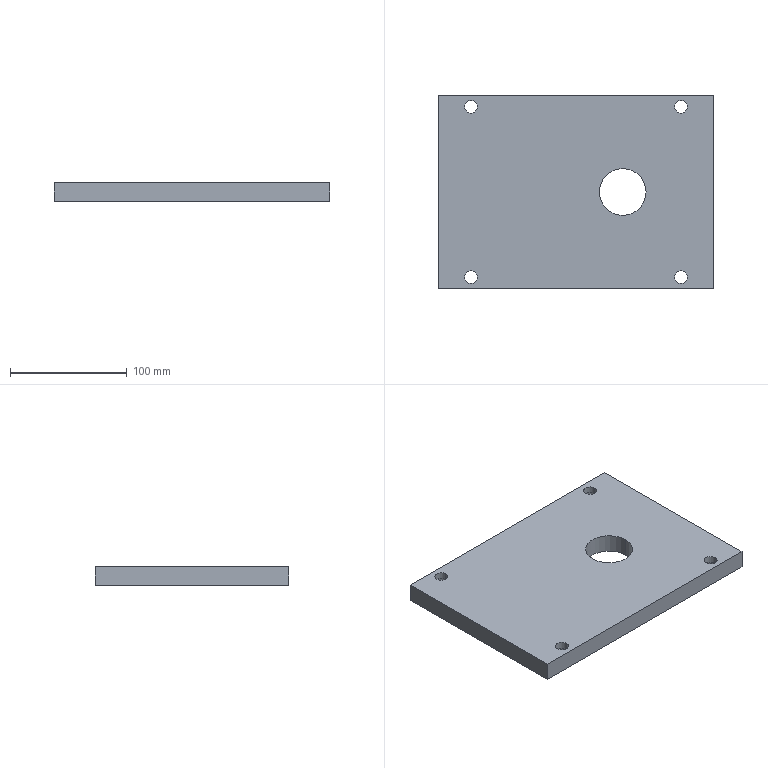Part | 1 solid | 28 faces | box 236 x 166 x 16 mm | volume 596387 mm3 | cylinder 18 | plane 10 | commonest cylinder face diameters 11 x8 16 x8 40 x2
STEP:
#1=CARTESIAN_POINT('',(60.,0.,-80.));
#2=VERTEX_POINT('',#1);
#3=CARTESIAN_POINT('',(20.,0.,-80.));
#4=VERTEX_POINT('',#3);
#5=CARTESIAN_POINT('',(40.,0.,-80.));
#6=DIRECTION('',(0.,0.,-1.));
#7=DIRECTION('',(-1.,0.,0.));
#8=AXIS2_PLACEMENT_3D('',#5,#6,#7);
#9=CIRCLE('',#8,20.);
#10=EDGE_CURVE('',#2,#4,#9,.T.);
#11=ORIENTED_EDGE('',*,*,#10,.F.);
#12=CARTESIAN_POINT('',(60.,0.,-96.));
#13=VERTEX_POINT('',#12);
#14=CARTESIAN_POINT('',(60.,0.,-80.));
#15=DIRECTION('',(0.,0.,-1.));
#16=VECTOR('',#15,1000.);
#17=LINE('',#14,#16);
#18=EDGE_CURVE('',#2,#13,#17,.T.);
#19=ORIENTED_EDGE('',*,*,#18,.T.);
#20=CARTESIAN_POINT('',(20.,0.,-96.));
#21=VERTEX_POINT('',#20);
#22=CARTESIAN_POINT('',(40.,0.,-96.));
#23=DIRECTION('',(0.,0.,1.));
#24=DIRECTION('',(-1.,0.,0.));
#25=AXIS2_PLACEMENT_3D('',#22,#23,#24);
#26=CIRCLE('',#25,20.);
#27=EDGE_CURVE('',#21,#13,#26,.T.);
#28=ORIENTED_EDGE('',*,*,#27,.F.);
#29=CARTESIAN_POINT('',(20.,0.,-80.));
#30=DIRECTION('',(0.,0.,-1.));
#31=VECTOR('',#30,1000.);
#32=LINE('',#29,#31);
#33=EDGE_CURVE('',#4,#21,#32,.T.);
#34=ORIENTED_EDGE('',*,*,#33,.F.);
#35=EDGE_LOOP('',(#11,#19,#28,#34));
#36=FACE_OUTER_BOUND('',#35,.T.);
#37=CARTESIAN_POINT('',(40.,0.,-80.));
#38=DIRECTION('',(0.,0.,-1.));
#39=DIRECTION('',(-1.,0.,0.));
#40=AXIS2_PLACEMENT_3D('',#37,#38,#39);
#41=CYLINDRICAL_SURFACE('',#40,20.);
#42=ADVANCED_FACE('',(#36),#41,.F.);
#43=CARTESIAN_POINT('',(-84.5,73.,-80.));
#44=VERTEX_POINT('',#43);
#45=CARTESIAN_POINT('',(-95.5,73.,-80.));
#46=VERTEX_POINT('',#45);
#47=CARTESIAN_POINT('',(-90.,73.,-80.));
#48=DIRECTION('',(0.,0.,-1.));
#49=DIRECTION('',(-1.,0.,0.));
#50=AXIS2_PLACEMENT_3D('',#47,#48,#49);
#51=CIRCLE('',#50,5.5);
#52=EDGE_CURVE('',#44,#46,#51,.T.);
#53=ORIENTED_EDGE('',*,*,#52,.F.);
#54=CARTESIAN_POINT('',(-84.5,73.,-86.));
#55=VERTEX_POINT('',#54);
#56=CARTESIAN_POINT('',(-84.5,73.,192.978));
#57=DIRECTION('',(0.,0.,-1.));
#58=VECTOR('',#57,1000.);
#59=LINE('',#56,#58);
#60=EDGE_CURVE('',#44,#55,#59,.T.);
#61=ORIENTED_EDGE('',*,*,#60,.T.);
#62=CARTESIAN_POINT('',(-95.5,73.,-86.));
#63=VERTEX_POINT('',#62);
#64=CARTESIAN_POINT('',(-90.,73.,-86.));
#65=DIRECTION('',(0.,0.,1.));
#66=DIRECTION('',(-1.,0.,0.));
#67=AXIS2_PLACEMENT_3D('',#64,#65,#66);
#68=CIRCLE('',#67,5.5);
#69=EDGE_CURVE('',#63,#55,#68,.T.);
#70=ORIENTED_EDGE('',*,*,#69,.F.);
#71=CARTESIAN_POINT('',(-95.5,73.,192.978));
#72=DIRECTION('',(0.,0.,-1.));
#73=VECTOR('',#72,1000.);
#74=LINE('',#71,#73);
#75=EDGE_CURVE('',#46,#63,#74,.T.);
#76=ORIENTED_EDGE('',*,*,#75,.F.);
#77=EDGE_LOOP('',(#53,#61,#70,#76));
#78=FACE_OUTER_BOUND('',#77,.T.);
#79=CARTESIAN_POINT('',(-90.,73.,192.978));
#80=DIRECTION('',(0.,0.,-1.));
#81=DIRECTION('',(-1.,0.,0.));
#82=AXIS2_PLACEMENT_3D('',#79,#80,#81);
#83=CYLINDRICAL_SURFACE('',#82,5.5);
#84=ADVANCED_FACE('',(#78),#83,.F.);
#85=CARTESIAN_POINT('',(95.5,-73.,-80.));
#86=VERTEX_POINT('',#85);
#87=CARTESIAN_POINT('',(84.5,-73.,-80.));
#88=VERTEX_POINT('',#87);
#89=CARTESIAN_POINT('',(90.,-73.,-80.));
#90=DIRECTION('',(0.,0.,-1.));
#91=DIRECTION('',(-1.,0.,0.));
#92=AXIS2_PLACEMENT_3D('',#89,#90,#91);
#93=CIRCLE('',#92,5.5);
#94=EDGE_CURVE('',#86,#88,#93,.T.);
#95=ORIENTED_EDGE('',*,*,#94,.F.);
#96=CARTESIAN_POINT('',(95.5,-73.,-86.));
#97=VERTEX_POINT('',#96);
#98=CARTESIAN_POINT('',(95.5,-73.,192.978));
#99=DIRECTION('',(0.,0.,-1.));
#100=VECTOR('',#99,1000.);
#101=LINE('',#98,#100);
#102=EDGE_CURVE('',#86,#97,#101,.T.);
#103=ORIENTED_EDGE('',*,*,#102,.T.);
#104=CARTESIAN_POINT('',(84.5,-73.,-86.));
#105=VERTEX_POINT('',#104);
#106=CARTESIAN_POINT('',(90.,-73.,-86.));
#107=DIRECTION('',(0.,0.,1.));
#108=DIRECTION('',(-1.,0.,0.));
#109=AXIS2_PLACEMENT_3D('',#106,#107,#108);
#110=CIRCLE('',#109,5.5);
#111=EDGE_CURVE('',#105,#97,#110,.T.);
#112=ORIENTED_EDGE('',*,*,#111,.F.);
#113=CARTESIAN_POINT('',(84.5,-73.,192.978));
#114=DIRECTION('',(0.,0.,-1.));
#115=VECTOR('',#114,1000.);
#116=LINE('',#113,#115);
#117=EDGE_CURVE('',#88,#105,#116,.T.);
#118=ORIENTED_EDGE('',*,*,#117,.F.);
#119=EDGE_LOOP('',(#95,#103,#112,#118));
#120=FACE_OUTER_BOUND('',#119,.T.);
#121=CARTESIAN_POINT('',(90.,-73.,192.978));
#122=DIRECTION('',(0.,0.,-1.));
#123=DIRECTION('',(-1.,0.,0.));
#124=AXIS2_PLACEMENT_3D('',#121,#122,#123);
#125=CYLINDRICAL_SURFACE('',#124,5.5);
#126=ADVANCED_FACE('',(#120),#125,.F.);
#127=CARTESIAN_POINT('',(95.5,73.,-80.));
#128=VERTEX_POINT('',#127);
#129=CARTESIAN_POINT('',(84.5,73.,-80.));
#130=VERTEX_POINT('',#129);
#131=CARTESIAN_POINT('',(90.,73.,-80.));
#132=DIRECTION('',(0.,0.,-1.));
#133=DIRECTION('',(-1.,0.,0.));
#134=AXIS2_PLACEMENT_3D('',#131,#132,#133);
#135=CIRCLE('',#134,5.5);
#136=EDGE_CURVE('',#128,#130,#135,.T.);
#137=ORIENTED_EDGE('',*,*,#136,.F.);
#138=CARTESIAN_POINT('',(95.5,73.,-86.));
#139=VERTEX_POINT('',#138);
#140=CARTESIAN_POINT('',(95.5,73.,192.978));
#141=DIRECTION('',(0.,0.,-1.));
#142=VECTOR('',#141,1000.);
#143=LINE('',#140,#142);
#144=EDGE_CURVE('',#128,#139,#143,.T.);
#145=ORIENTED_EDGE('',*,*,#144,.T.);
#146=CARTESIAN_POINT('',(84.5,73.,-86.));
#147=VERTEX_POINT('',#146);
#148=CARTESIAN_POINT('',(90.,73.,-86.));
#149=DIRECTION('',(0.,0.,1.));
#150=DIRECTION('',(-1.,0.,0.));
#151=AXIS2_PLACEMENT_3D('',#148,#149,#150);
#152=CIRCLE('',#151,5.5);
#153=EDGE_CURVE('',#147,#139,#152,.T.);
#154=ORIENTED_EDGE('',*,*,#153,.F.);
#155=CARTESIAN_POINT('',(84.5,73.,192.978));
#156=DIRECTION('',(0.,0.,-1.));
#157=VECTOR('',#156,1000.);
#158=LINE('',#155,#157);
#159=EDGE_CURVE('',#130,#147,#158,.T.);
#160=ORIENTED_EDGE('',*,*,#159,.F.);
#161=EDGE_LOOP('',(#137,#145,#154,#160));
#162=FACE_OUTER_BOUND('',#161,.T.);
#163=CARTESIAN_POINT('',(90.,73.,192.978));
#164=DIRECTION('',(0.,0.,-1.));
#165=DIRECTION('',(-1.,0.,0.));
#166=AXIS2_PLACEMENT_3D('',#163,#164,#165);
#167=CYLINDRICAL_SURFACE('',#166,5.5);
#168=ADVANCED_FACE('',(#162),#167,.F.);
#169=CARTESIAN_POINT('',(-84.5,-73.,-80.));
#170=VERTEX_POINT('',#169);
#171=CARTESIAN_POINT('',(-95.5,-73.,-80.));
#172=VERTEX_POINT('',#171);
#173=CARTESIAN_POINT('',(-90.,-73.,-80.));
#174=DIRECTION('',(0.,0.,-1.));
#175=DIRECTION('',(-1.,0.,0.));
#176=AXIS2_PLACEMENT_3D('',#173,#174,#175);
#177=CIRCLE('',#176,5.5);
#178=EDGE_CURVE('',#170,#172,#177,.T.);
#179=ORIENTED_EDGE('',*,*,#178,.F.);
#180=CARTESIAN_POINT('',(-84.5,-73.,-86.));
#181=VERTEX_POINT('',#180);
#182=CARTESIAN_POINT('',(-84.5,-73.,192.978));
#183=DIRECTION('',(0.,0.,-1.));
#184=VECTOR('',#183,1000.);
#185=LINE('',#182,#184);
#186=EDGE_CURVE('',#170,#181,#185,.T.);
#187=ORIENTED_EDGE('',*,*,#186,.T.);
#188=CARTESIAN_POINT('',(-95.5,-73.,-86.));
#189=VERTEX_POINT('',#188);
#190=CARTESIAN_POINT('',(-90.,-73.,-86.));
#191=DIRECTION('',(0.,0.,1.));
#192=DIRECTION('',(-1.,0.,0.));
#193=AXIS2_PLACEMENT_3D('',#190,#191,#192);
#194=CIRCLE('',#193,5.5);
#195=EDGE_CURVE('',#189,#181,#194,.T.);
#196=ORIENTED_EDGE('',*,*,#195,.F.);
#197=CARTESIAN_POINT('',(-95.5,-73.,192.978));
#198=DIRECTION('',(0.,0.,-1.));
#199=VECTOR('',#198,1000.);
#200=LINE('',#197,#199);
#201=EDGE_CURVE('',#172,#189,#200,.T.);
#202=ORIENTED_EDGE('',*,*,#201,.F.);
#203=EDGE_LOOP('',(#179,#187,#196,#202));
#204=FACE_OUTER_BOUND('',#203,.T.);
#205=CARTESIAN_POINT('',(-90.,-73.,192.978));
#206=DIRECTION('',(0.,0.,-1.));
#207=DIRECTION('',(-1.,0.,0.));
#208=AXIS2_PLACEMENT_3D('',#205,#206,#207);
#209=CYLINDRICAL_SURFACE('',#208,5.5);
#210=ADVANCED_FACE('',(#204),#209,.F.);
#211=CARTESIAN_POINT('',(-82.,73.,-86.));
#212=VERTEX_POINT('',#211);
#213=CARTESIAN_POINT('',(-98.,73.,-86.));
#214=VERTEX_POINT('',#213);
#215=CARTESIAN_POINT('',(-90.,73.,-86.));
#216=DIRECTION('',(0.,0.,-1.));
#217=DIRECTION('',(-1.,0.,0.));
#218=AXIS2_PLACEMENT_3D('',#215,#216,#217);
#219=CIRCLE('',#218,8.);
#220=EDGE_CURVE('',#212,#214,#219,.T.);
#221=ORIENTED_EDGE('',*,*,#220,.F.);
#222=CARTESIAN_POINT('',(-82.,73.,-96.));
#223=VERTEX_POINT('',#222);
#224=CARTESIAN_POINT('',(-82.,73.,-91.));
#225=DIRECTION('',(0.,0.,-1.));
#226=VECTOR('',#225,1000.);
#227=LINE('',#224,#226);
#228=EDGE_CURVE('',#212,#223,#227,.T.);
#229=ORIENTED_EDGE('',*,*,#228,.T.);
#230=CARTESIAN_POINT('',(-98.,73.,-96.));
#231=VERTEX_POINT('',#230);
#232=CARTESIAN_POINT('',(-90.,73.,-96.));
#233=DIRECTION('',(0.,0.,1.));
#234=DIRECTION('',(-1.,0.,0.));
#235=AXIS2_PLACEMENT_3D('',#232,#233,#234);
#236=CIRCLE('',#235,8.);
#237=EDGE_CURVE('',#231,#223,#236,.T.);
#238=ORIENTED_EDGE('',*,*,#237,.F.);
#239=CARTESIAN_POINT('',(-98.,73.,-91.));
#240=DIRECTION('',(0.,0.,-1.));
#241=VECTOR('',#240,1000.);
#242=LINE('',#239,#241);
#243=EDGE_CURVE('',#214,#231,#242,.T.);
#244=ORIENTED_EDGE('',*,*,#243,.F.);
#245=EDGE_LOOP('',(#221,#229,#238,#244));
#246=FACE_OUTER_BOUND('',#245,.T.);
#247=CARTESIAN_POINT('',(-90.,73.,-91.));
#248=DIRECTION('',(0.,0.,-1.));
#249=DIRECTION('',(-1.,0.,0.));
#250=AXIS2_PLACEMENT_3D('',#247,#248,#249);
#251=CYLINDRICAL_SURFACE('',#250,8.);
#252=ADVANCED_FACE('',(#246),#251,.F.);
#253=CARTESIAN_POINT('',(98.,-73.,-86.));
#254=VERTEX_POINT('',#253);
#255=CARTESIAN_POINT('',(82.,-73.,-86.));
#256=VERTEX_POINT('',#255);
#257=CARTESIAN_POINT('',(90.,-73.,-86.));
#258=DIRECTION('',(0.,0.,-1.));
#259=DIRECTION('',(-1.,0.,0.));
#260=AXIS2_PLACEMENT_3D('',#257,#258,#259);
#261=CIRCLE('',#260,8.);
#262=EDGE_CURVE('',#254,#256,#261,.T.);
#263=ORIENTED_EDGE('',*,*,#262,.F.);
#264=CARTESIAN_POINT('',(98.,-73.,-96.));
#265=VERTEX_POINT('',#264);
#266=CARTESIAN_POINT('',(98.,-73.,-91.));
#267=DIRECTION('',(0.,0.,-1.));
#268=VECTOR('',#267,1000.);
#269=LINE('',#266,#268);
#270=EDGE_CURVE('',#254,#265,#269,.T.);
#271=ORIENTED_EDGE('',*,*,#270,.T.);
#272=CARTESIAN_POINT('',(82.,-73.,-96.));
#273=VERTEX_POINT('',#272);
#274=CARTESIAN_POINT('',(90.,-73.,-96.));
#275=DIRECTION('',(0.,0.,1.));
#276=DIRECTION('',(-1.,0.,0.));
#277=AXIS2_PLACEMENT_3D('',#274,#275,#276);
#278=CIRCLE('',#277,8.);
#279=EDGE_CURVE('',#273,#265,#278,.T.);
#280=ORIENTED_EDGE('',*,*,#279,.F.);
#281=CARTESIAN_POINT('',(82.,-73.,-91.));
#282=DIRECTION('',(0.,0.,-1.));
#283=VECTOR('',#282,1000.);
#284=LINE('',#281,#283);
#285=EDGE_CURVE('',#256,#273,#284,.T.);
#286=ORIENTED_EDGE('',*,*,#285,.F.);
#287=EDGE_LOOP('',(#263,#271,#280,#286));
#288=FACE_OUTER_BOUND('',#287,.T.);
#289=CARTESIAN_POINT('',(90.,-73.,-91.));
#290=DIRECTION('',(0.,0.,-1.));
#291=DIRECTION('',(-1.,0.,0.));
#292=AXIS2_PLACEMENT_3D('',#289,#290,#291);
#293=CYLINDRICAL_SURFACE('',#292,8.);
#294=ADVANCED_FACE('',(#288),#293,.F.);
#295=CARTESIAN_POINT('',(98.,73.,-86.));
#296=VERTEX_POINT('',#295);
#297=CARTESIAN_POINT('',(82.,73.,-86.));
#298=VERTEX_POINT('',#297);
#299=CARTESIAN_POINT('',(90.,73.,-86.));
#300=DIRECTION('',(0.,0.,-1.));
#301=DIRECTION('',(-1.,0.,0.));
#302=AXIS2_PLACEMENT_3D('',#299,#300,#301);
#303=CIRCLE('',#302,8.);
#304=EDGE_CURVE('',#296,#298,#303,.T.);
#305=ORIENTED_EDGE('',*,*,#304,.F.);
#306=CARTESIAN_POINT('',(98.,73.,-96.));
#307=VERTEX_POINT('',#306);
#308=CARTESIAN_POINT('',(98.,73.,-91.));
#309=DIRECTION('',(0.,0.,-1.));
#310=VECTOR('',#309,1000.);
#311=LINE('',#308,#310);
#312=EDGE_CURVE('',#296,#307,#311,.T.);
#313=ORIENTED_EDGE('',*,*,#312,.T.);
#314=CARTESIAN_POINT('',(82.,73.,-96.));
#315=VERTEX_POINT('',#314);
#316=CARTESIAN_POINT('',(90.,73.,-96.));
#317=DIRECTION('',(0.,0.,1.));
#318=DIRECTION('',(-1.,0.,0.));
#319=AXIS2_PLACEMENT_3D('',#316,#317,#318);
#320=CIRCLE('',#319,8.);
#321=EDGE_CURVE('',#315,#307,#320,.T.);
#322=ORIENTED_EDGE('',*,*,#321,.F.);
#323=CARTESIAN_POINT('',(82.,73.,-91.));
#324=DIRECTION('',(0.,0.,-1.));
#325=VECTOR('',#324,1000.);
#326=LINE('',#323,#325);
#327=EDGE_CURVE('',#298,#315,#326,.T.);
#328=ORIENTED_EDGE('',*,*,#327,.F.);
#329=EDGE_LOOP('',(#305,#313,#322,#328));
#330=FACE_OUTER_BOUND('',#329,.T.);
#331=CARTESIAN_POINT('',(90.,73.,-91.));
#332=DIRECTION('',(0.,0.,-1.));
#333=DIRECTION('',(-1.,0.,0.));
#334=AXIS2_PLACEMENT_3D('',#331,#332,#333);
#335=CYLINDRICAL_SURFACE('',#334,8.);
#336=ADVANCED_FACE('',(#330),#335,.F.);
#337=CARTESIAN_POINT('',(-82.,-73.,-86.));
#338=VERTEX_POINT('',#337);
#339=CARTESIAN_POINT('',(-98.,-73.,-86.));
#340=VERTEX_POINT('',#339);
#341=CARTESIAN_POINT('',(-90.,-73.,-86.));
#342=DIRECTION('',(0.,0.,-1.));
#343=DIRECTION('',(-1.,0.,0.));
#344=AXIS2_PLACEMENT_3D('',#341,#342,#343);
#345=CIRCLE('',#344,8.);
#346=EDGE_CURVE('',#338,#340,#345,.T.);
#347=ORIENTED_EDGE('',*,*,#346,.F.);
#348=CARTESIAN_POINT('',(-82.,-73.,-96.));
#349=VERTEX_POINT('',#348);
#350=CARTESIAN_POINT('',(-82.,-73.,-91.));
#351=DIRECTION('',(0.,0.,-1.));
#352=VECTOR('',#351,1000.);
#353=LINE('',#350,#352);
#354=EDGE_CURVE('',#338,#349,#353,.T.);
#355=ORIENTED_EDGE('',*,*,#354,.T.);
#356=CARTESIAN_POINT('',(-98.,-73.,-96.));
#357=VERTEX_POINT('',#356);
#358=CARTESIAN_POINT('',(-90.,-73.,-96.));
#359=DIRECTION('',(0.,0.,1.));
#360=DIRECTION('',(-1.,0.,0.));
#361=AXIS2_PLACEMENT_3D('',#358,#359,#360);
#362=CIRCLE('',#361,8.);
#363=EDGE_CURVE('',#357,#349,#362,.T.);
#364=ORIENTED_EDGE('',*,*,#363,.F.);
#365=CARTESIAN_POINT('',(-98.,-73.,-91.));
#366=DIRECTION('',(0.,0.,-1.));
#367=VECTOR('',#366,1000.);
#368=LINE('',#365,#367);
#369=EDGE_CURVE('',#340,#357,#368,.T.);
#370=ORIENTED_EDGE('',*,*,#369,.F.);
#371=EDGE_LOOP('',(#347,#355,#364,#370));
#372=FACE_OUTER_BOUND('',#371,.T.);
#373=CARTESIAN_POINT('',(-90.,-73.,-91.));
#374=DIRECTION('',(0.,0.,-1.));
#375=DIRECTION('',(-1.,0.,0.));
#376=AXIS2_PLACEMENT_3D('',#373,#374,#375);
#377=CYLINDRICAL_SURFACE('',#376,8.);
#378=ADVANCED_FACE('',(#372),#377,.F.);
#379=CARTESIAN_POINT('',(40.,0.,-80.));
#380=DIRECTION('',(0.,0.,-1.));
#381=DIRECTION('',(-1.,0.,0.));
#382=AXIS2_PLACEMENT_3D('',#379,#380,#381);
#383=CIRCLE('',#382,20.);
#384=EDGE_CURVE('',#4,#2,#383,.T.);
#385=ORIENTED_EDGE('',*,*,#384,.T.);
#386=ORIENTED_EDGE('',*,*,#10,.T.);
#387=EDGE_LOOP('',(#385,#386));
#388=FACE_BOUND('',#387,.T.);
#389=CARTESIAN_POINT('',(-90.,73.,-80.));
#390=DIRECTION('',(0.,0.,-1.));
#391=DIRECTION('',(-1.,0.,0.));
#392=AXIS2_PLACEMENT_3D('',#389,#390,#391);
#393=CIRCLE('',#392,5.5);
#394=EDGE_CURVE('',#46,#44,#393,.T.);
#395=ORIENTED_EDGE('',*,*,#394,.T.);
#396=ORIENTED_EDGE('',*,*,#52,.T.);
#397=EDGE_LOOP('',(#395,#396));
#398=FACE_BOUND('',#397,.T.);
#399=CARTESIAN_POINT('',(90.,-73.,-80.));
#400=DIRECTION('',(0.,0.,-1.));
#401=DIRECTION('',(-1.,0.,0.));
#402=AXIS2_PLACEMENT_3D('',#399,#400,#401);
#403=CIRCLE('',#402,5.5);
#404=EDGE_CURVE('',#88,#86,#403,.T.);
#405=ORIENTED_EDGE('',*,*,#404,.T.);
#406=ORIENTED_EDGE('',*,*,#94,.T.);
#407=EDGE_LOOP('',(#405,#406));
#408=FACE_BOUND('',#407,.T.);
#409=CARTESIAN_POINT('',(90.,73.,-80.));
#410=DIRECTION('',(0.,0.,-1.));
#411=DIRECTION('',(-1.,0.,0.));
#412=AXIS2_PLACEMENT_3D('',#409,#410,#411);
#413=CIRCLE('',#412,5.5);
#414=EDGE_CURVE('',#130,#128,#413,.T.);
#415=ORIENTED_EDGE('',*,*,#414,.T.);
#416=ORIENTED_EDGE('',*,*,#136,.T.);
#417=EDGE_LOOP('',(#415,#416));
#418=FACE_BOUND('',#417,.T.);
#419=CARTESIAN_POINT('',(-90.,-73.,-80.));
#420=DIRECTION('',(0.,0.,-1.));
#421=DIRECTION('',(-1.,0.,0.));
#422=AXIS2_PLACEMENT_3D('',#419,#420,#421);
#423=CIRCLE('',#422,5.5);
#424=EDGE_CURVE('',#172,#170,#423,.T.);
#425=ORIENTED_EDGE('',*,*,#424,.T.);
#426=ORIENTED_EDGE('',*,*,#178,.T.);
#427=EDGE_LOOP('',(#425,#426));
#428=FACE_BOUND('',#427,.T.);
#429=CARTESIAN_POINT('',(-118.,-83.,-80.));
#430=VERTEX_POINT('',#429);
#431=CARTESIAN_POINT('',(118.,-83.,-80.));
#432=VERTEX_POINT('',#431);
#433=CARTESIAN_POINT('',(0.,-83.,-80.));
#434=DIRECTION('',(1.,0.,0.));
#435=VECTOR('',#434,1000.);
#436=LINE('',#433,#435);
#437=EDGE_CURVE('',#430,#432,#436,.T.);
#438=ORIENTED_EDGE('',*,*,#437,.T.);
#439=CARTESIAN_POINT('',(118.,83.,-80.));
#440=VERTEX_POINT('',#439);
#441=CARTESIAN_POINT('',(118.,0.,-80.));
#442=DIRECTION('',(0.,1.,0.));
#443=VECTOR('',#442,1000.);
#444=LINE('',#441,#443);
#445=EDGE_CURVE('',#432,#440,#444,.T.);
#446=ORIENTED_EDGE('',*,*,#445,.T.);
#447=CARTESIAN_POINT('',(-118.,83.,-80.));
#448=VERTEX_POINT('',#447);
#449=CARTESIAN_POINT('',(0.,83.,-80.));
#450=DIRECTION('',(-1.,0.,0.));
#451=VECTOR('',#450,1000.);
#452=LINE('',#449,#451);
#453=EDGE_CURVE('',#440,#448,#452,.T.);
#454=ORIENTED_EDGE('',*,*,#453,.T.);
#455=CARTESIAN_POINT('',(-118.,0.,-80.));
#456=DIRECTION('',(0.,-1.,0.));
#457=VECTOR('',#456,1000.);
#458=LINE('',#455,#457);
#459=EDGE_CURVE('',#448,#430,#458,.T.);
#460=ORIENTED_EDGE('',*,*,#459,.T.);
#461=EDGE_LOOP('',(#438,#446,#454,#460));
#462=FACE_OUTER_BOUND('',#461,.T.);
#463=CARTESIAN_POINT('',(0.,0.,-80.));
#464=DIRECTION('',(0.,0.,1.));
#465=DIRECTION('',(1.,0.,0.));
#466=AXIS2_PLACEMENT_3D('',#463,#464,#465);
#467=PLANE('',#466);
#468=ADVANCED_FACE('',(#388,#398,#408,#418,#428,#462),#467,.T.);
#469=ORIENTED_EDGE('',*,*,#18,.F.);
#470=ORIENTED_EDGE('',*,*,#384,.F.);
#471=ORIENTED_EDGE('',*,*,#33,.T.);
#472=CARTESIAN_POINT('',(40.,0.,-96.));
#473=DIRECTION('',(0.,0.,1.));
#474=DIRECTION('',(-1.,0.,0.));
#475=AXIS2_PLACEMENT_3D('',#472,#473,#474);
#476=CIRCLE('',#475,20.);
#477=EDGE_CURVE('',#13,#21,#476,.T.);
#478=ORIENTED_EDGE('',*,*,#477,.F.);
#479=EDGE_LOOP('',(#469,#470,#471,#478));
#480=FACE_OUTER_BOUND('',#479,.T.);
#481=CARTESIAN_POINT('',(40.,0.,-80.));
#482=DIRECTION('',(0.,0.,-1.));
#483=DIRECTION('',(-1.,0.,0.));
#484=AXIS2_PLACEMENT_3D('',#481,#482,#483);
#485=CYLINDRICAL_SURFACE('',#484,20.);
#486=ADVANCED_FACE('',(#480),#485,.F.);
#487=ORIENTED_EDGE('',*,*,#60,.F.);
#488=ORIENTED_EDGE('',*,*,#394,.F.);
#489=ORIENTED_EDGE('',*,*,#75,.T.);
#490=CARTESIAN_POINT('',(-90.,73.,-86.));
#491=DIRECTION('',(0.,0.,1.));
#492=DIRECTION('',(-1.,0.,0.));
#493=AXIS2_PLACEMENT_3D('',#490,#491,#492);
#494=CIRCLE('',#493,5.5);
#495=EDGE_CURVE('',#55,#63,#494,.T.);
#496=ORIENTED_EDGE('',*,*,#495,.F.);
#497=EDGE_LOOP('',(#487,#488,#489,#496));
#498=FACE_OUTER_BOUND('',#497,.T.);
#499=CARTESIAN_POINT('',(-90.,73.,192.978));
#500=DIRECTION('',(0.,0.,-1.));
#501=DIRECTION('',(-1.,0.,0.));
#502=AXIS2_PLACEMENT_3D('',#499,#500,#501);
#503=CYLINDRICAL_SURFACE('',#502,5.5);
#504=ADVANCED_FACE('',(#498),#503,.F.);
#505=ORIENTED_EDGE('',*,*,#102,.F.);
#506=ORIENTED_EDGE('',*,*,#404,.F.);
#507=ORIENTED_EDGE('',*,*,#117,.T.);
#508=CARTESIAN_POINT('',(90.,-73.,-86.));
#509=DIRECTION('',(0.,0.,1.));
#510=DIRECTION('',(-1.,0.,0.));
#511=AXIS2_PLACEMENT_3D('',#508,#509,#510);
#512=CIRCLE('',#511,5.5);
#513=EDGE_CURVE('',#97,#105,#512,.T.);
#514=ORIENTED_EDGE('',*,*,#513,.F.);
#515=EDGE_LOOP('',(#505,#506,#507,#514));
#516=FACE_OUTER_BOUND('',#515,.T.);
#517=CARTESIAN_POINT('',(90.,-73.,192.978));
#518=DIRECTION('',(0.,0.,-1.));
#519=DIRECTION('',(-1.,0.,0.));
#520=AXIS2_PLACEMENT_3D('',#517,#518,#519);
#521=CYLINDRICAL_SURFACE('',#520,5.5);
#522=ADVANCED_FACE('',(#516),#521,.F.);
#523=ORIENTED_EDGE('',*,*,#144,.F.);
#524=ORIENTED_EDGE('',*,*,#414,.F.);
#525=ORIENTED_EDGE('',*,*,#159,.T.);
#526=CARTESIAN_POINT('',(90.,73.,-86.));
#527=DIRECTION('',(0.,0.,1.));
#528=DIRECTION('',(-1.,0.,0.));
#529=AXIS2_PLACEMENT_3D('',#526,#527,#528);
#530=CIRCLE('',#529,5.5);
#531=EDGE_CURVE('',#139,#147,#530,.T.);
#532=ORIENTED_EDGE('',*,*,#531,.F.);
#533=EDGE_LOOP('',(#523,#524,#525,#532));
#534=FACE_OUTER_BOUND('',#533,.T.);
#535=CARTESIAN_POINT('',(90.,73.,192.978));
#536=DIRECTION('',(0.,0.,-1.));
#537=DIRECTION('',(-1.,0.,0.));
#538=AXIS2_PLACEMENT_3D('',#535,#536,#537);
#539=CYLINDRICAL_SURFACE('',#538,5.5);
#540=ADVANCED_FACE('',(#534),#539,.F.);
#541=ORIENTED_EDGE('',*,*,#186,.F.);
#542=ORIENTED_EDGE('',*,*,#424,.F.);
#543=ORIENTED_EDGE('',*,*,#201,.T.);
#544=CARTESIAN_POINT('',(-90.,-73.,-86.));
#545=DIRECTION('',(0.,0.,1.));
#546=DIRECTION('',(-1.,0.,0.));
#547=AXIS2_PLACEMENT_3D('',#544,#545,#546);
#548=CIRCLE('',#547,5.5);
#549=EDGE_CURVE('',#181,#189,#548,.T.);
#550=ORIENTED_EDGE('',*,*,#549,.F.);
#551=EDGE_LOOP('',(#541,#542,#543,#550));
#552=FACE_OUTER_BOUND('',#551,.T.);
#553=CARTESIAN_POINT('',(-90.,-73.,192.978));
#554=DIRECTION('',(0.,0.,-1.));
#555=DIRECTION('',(-1.,0.,0.));
#556=AXIS2_PLACEMENT_3D('',#553,#554,#555);
#557=CYLINDRICAL_SURFACE('',#556,5.5);
#558=ADVANCED_FACE('',(#552),#557,.F.);
#559=CARTESIAN_POINT('',(118.,-83.,-96.));
#560=VERTEX_POINT('',#559);
#561=CARTESIAN_POINT('',(118.,83.,-96.));
#562=VERTEX_POINT('',#561);
#563=CARTESIAN_POINT('',(118.,83.,-96.));
#564=DIRECTION('',(0.,1.,0.));
#565=VECTOR('',#564,1000.);
#566=LINE('',#563,#565);
#567=EDGE_CURVE('',#560,#562,#566,.T.);
#568=ORIENTED_EDGE('',*,*,#567,.T.);
#569=CARTESIAN_POINT('',(118.,83.,-80.));
#570=DIRECTION('',(0.,0.,1.));
#571=VECTOR('',#570,1000.);
#572=LINE('',#569,#571);
#573=EDGE_CURVE('',#562,#440,#572,.T.);
#574=ORIENTED_EDGE('',*,*,#573,.T.);
#575=ORIENTED_EDGE('',*,*,#445,.F.);
#576=CARTESIAN_POINT('',(118.,-83.,-80.));
#577=DIRECTION('',(0.,0.,-1.));
#578=VECTOR('',#577,1000.);
#579=LINE('',#576,#578);
#580=EDGE_CURVE('',#432,#560,#579,.T.);
#581=ORIENTED_EDGE('',*,*,#580,.T.);
#582=EDGE_LOOP('',(#568,#574,#575,#581));
#583=FACE_OUTER_BOUND('',#582,.T.);
#584=CARTESIAN_POINT('',(118.,83.,-80.));
#585=DIRECTION('',(1.,0.,0.));
#586=DIRECTION('',(0.,1.,0.));
#587=AXIS2_PLACEMENT_3D('',#584,#585,#586);
#588=PLANE('',#587);
#589=ADVANCED_FACE('',(#583),#588,.T.);
#590=CARTESIAN_POINT('',(-118.,-83.,-96.));
#591=VERTEX_POINT('',#590);
#592=CARTESIAN_POINT('',(118.,-83.,-96.));
#593=DIRECTION('',(1.,0.,0.));
#594=VECTOR('',#593,1000.);
#595=LINE('',#592,#594);
#596=EDGE_CURVE('',#591,#560,#595,.T.);
#597=ORIENTED_EDGE('',*,*,#596,.T.);
#598=ORIENTED_EDGE('',*,*,#580,.F.);
#599=ORIENTED_EDGE('',*,*,#437,.F.);
#600=CARTESIAN_POINT('',(-118.,-83.,-80.));
#601=DIRECTION('',(0.,0.,-1.));
#602=VECTOR('',#601,1000.);
#603=LINE('',#600,#602);
#604=EDGE_CURVE('',#430,#591,#603,.T.);
#605=ORIENTED_EDGE('',*,*,#604,.T.);
#606=EDGE_LOOP('',(#597,#598,#599,#605));
#607=FACE_OUTER_BOUND('',#606,.T.);
#608=CARTESIAN_POINT('',(118.,-83.,-80.));
#609=DIRECTION('',(0.,-1.,0.));
#610=DIRECTION('',(1.,0.,0.));
#611=AXIS2_PLACEMENT_3D('',#608,#609,#610);
#612=PLANE('',#611);
#613=ADVANCED_FACE('',(#607),#612,.T.);
#614=CARTESIAN_POINT('',(-118.,83.,-96.));
#615=VERTEX_POINT('',#614);
#616=CARTESIAN_POINT('',(-118.,-83.,-96.));
#617=DIRECTION('',(0.,-1.,0.));
#618=VECTOR('',#617,1000.);
#619=LINE('',#616,#618);
#620=EDGE_CURVE('',#615,#591,#619,.T.);
#621=ORIENTED_EDGE('',*,*,#620,.T.);
#622=ORIENTED_EDGE('',*,*,#604,.F.);
#623=ORIENTED_EDGE('',*,*,#459,.F.);
#624=CARTESIAN_POINT('',(-118.,83.,-80.));
#625=DIRECTION('',(0.,0.,-1.));
#626=VECTOR('',#625,1000.);
#627=LINE('',#624,#626);
#628=EDGE_CURVE('',#448,#615,#627,.T.);
#629=ORIENTED_EDGE('',*,*,#628,.T.);
#630=EDGE_LOOP('',(#621,#622,#623,#629));
#631=FACE_OUTER_BOUND('',#630,.T.);
#632=CARTESIAN_POINT('',(-118.,-83.,-80.));
#633=DIRECTION('',(-1.,0.,0.));
#634=DIRECTION('',(0.,-1.,0.));
#635=AXIS2_PLACEMENT_3D('',#632,#633,#634);
#636=PLANE('',#635);
#637=ADVANCED_FACE('',(#631),#636,.T.);
#638=CARTESIAN_POINT('',(-118.,83.,-96.));
#639=DIRECTION('',(-1.,0.,0.));
#640=VECTOR('',#639,1000.);
#641=LINE('',#638,#640);
#642=EDGE_CURVE('',#562,#615,#641,.T.);
#643=ORIENTED_EDGE('',*,*,#642,.T.);
#644=ORIENTED_EDGE('',*,*,#628,.F.);
#645=ORIENTED_EDGE('',*,*,#453,.F.);
#646=ORIENTED_EDGE('',*,*,#573,.F.);
#647=EDGE_LOOP('',(#643,#644,#645,#646));
#648=FACE_OUTER_BOUND('',#647,.T.);
#649=CARTESIAN_POINT('',(-118.,83.,-80.));
#650=DIRECTION('',(0.,1.,0.));
#651=DIRECTION('',(0.,0.,1.));
#652=AXIS2_PLACEMENT_3D('',#649,#650,#651);
#653=PLANE('',#652);
#654=ADVANCED_FACE('',(#648),#653,.T.);
#655=ORIENTED_EDGE('',*,*,#27,.T.);
#656=ORIENTED_EDGE('',*,*,#477,.T.);
#657=EDGE_LOOP('',(#655,#656));
#658=FACE_BOUND('',#657,.T.);
#659=ORIENTED_EDGE('',*,*,#237,.T.);
#660=CARTESIAN_POINT('',(-90.,73.,-96.));
#661=DIRECTION('',(0.,0.,1.));
#662=DIRECTION('',(-1.,0.,0.));
#663=AXIS2_PLACEMENT_3D('',#660,#661,#662);
#664=CIRCLE('',#663,8.);
#665=EDGE_CURVE('',#223,#231,#664,.T.);
#666=ORIENTED_EDGE('',*,*,#665,.T.);
#667=EDGE_LOOP('',(#659,#666));
#668=FACE_BOUND('',#667,.T.);
#669=ORIENTED_EDGE('',*,*,#279,.T.);
#670=CARTESIAN_POINT('',(90.,-73.,-96.));
#671=DIRECTION('',(0.,0.,1.));
#672=DIRECTION('',(-1.,0.,0.));
#673=AXIS2_PLACEMENT_3D('',#670,#671,#672);
#674=CIRCLE('',#673,8.);
#675=EDGE_CURVE('',#265,#273,#674,.T.);
#676=ORIENTED_EDGE('',*,*,#675,.T.);
#677=EDGE_LOOP('',(#669,#676));
#678=FACE_BOUND('',#677,.T.);
#679=ORIENTED_EDGE('',*,*,#321,.T.);
#680=CARTESIAN_POINT('',(90.,73.,-96.));
#681=DIRECTION('',(0.,0.,1.));
#682=DIRECTION('',(-1.,0.,0.));
#683=AXIS2_PLACEMENT_3D('',#680,#681,#682);
#684=CIRCLE('',#683,8.);
#685=EDGE_CURVE('',#307,#315,#684,.T.);
#686=ORIENTED_EDGE('',*,*,#685,.T.);
#687=EDGE_LOOP('',(#679,#686));
#688=FACE_BOUND('',#687,.T.);
#689=ORIENTED_EDGE('',*,*,#363,.T.);
#690=CARTESIAN_POINT('',(-90.,-73.,-96.));
#691=DIRECTION('',(0.,0.,1.));
#692=DIRECTION('',(-1.,0.,0.));
#693=AXIS2_PLACEMENT_3D('',#690,#691,#692);
#694=CIRCLE('',#693,8.);
#695=EDGE_CURVE('',#349,#357,#694,.T.);
#696=ORIENTED_EDGE('',*,*,#695,.T.);
#697=EDGE_LOOP('',(#689,#696));
#698=FACE_BOUND('',#697,.T.);
#699=ORIENTED_EDGE('',*,*,#596,.F.);
#700=ORIENTED_EDGE('',*,*,#620,.F.);
#701=ORIENTED_EDGE('',*,*,#642,.F.);
#702=ORIENTED_EDGE('',*,*,#567,.F.);
#703=EDGE_LOOP('',(#699,#700,#701,#702));
#704=FACE_OUTER_BOUND('',#703,.T.);
#705=CARTESIAN_POINT('',(0.,0.,-96.));
#706=DIRECTION('',(0.,0.,-1.));
#707=DIRECTION('',(-1.,0.,0.));
#708=AXIS2_PLACEMENT_3D('',#705,#706,#707);
#709=PLANE('',#708);
#710=ADVANCED_FACE('',(#658,#668,#678,#688,#698,#704),#709,.T.);
#711=ORIENTED_EDGE('',*,*,#69,.T.);
#712=ORIENTED_EDGE('',*,*,#495,.T.);
#713=EDGE_LOOP('',(#711,#712));
#714=FACE_BOUND('',#713,.T.);
#715=CARTESIAN_POINT('',(-90.,73.,-86.));
#716=DIRECTION('',(0.,0.,-1.));
#717=DIRECTION('',(-1.,0.,0.));
#718=AXIS2_PLACEMENT_3D('',#715,#716,#717);
#719=CIRCLE('',#718,8.);
#720=EDGE_CURVE('',#214,#212,#719,.T.);
#721=ORIENTED_EDGE('',*,*,#720,.T.);
#722=ORIENTED_EDGE('',*,*,#220,.T.);
#723=EDGE_LOOP('',(#721,#722));
#724=FACE_OUTER_BOUND('',#723,.T.);
#725=CARTESIAN_POINT('',(-90.,73.,-86.));
#726=DIRECTION('',(0.,0.,-1.));
#727=DIRECTION('',(-1.,0.,0.));
#728=AXIS2_PLACEMENT_3D('',#725,#726,#727);
#729=PLANE('',#728);
#730=ADVANCED_FACE('',(#714,#724),#729,.T.);
#731=ORIENTED_EDGE('',*,*,#111,.T.);
#732=ORIENTED_EDGE('',*,*,#513,.T.);
#733=EDGE_LOOP('',(#731,#732));
#734=FACE_BOUND('',#733,.T.);
#735=CARTESIAN_POINT('',(90.,-73.,-86.));
#736=DIRECTION('',(0.,0.,-1.));
#737=DIRECTION('',(-1.,0.,0.));
#738=AXIS2_PLACEMENT_3D('',#735,#736,#737);
#739=CIRCLE('',#738,8.);
#740=EDGE_CURVE('',#256,#254,#739,.T.);
#741=ORIENTED_EDGE('',*,*,#740,.T.);
#742=ORIENTED_EDGE('',*,*,#262,.T.);
#743=EDGE_LOOP('',(#741,#742));
#744=FACE_OUTER_BOUND('',#743,.T.);
#745=CARTESIAN_POINT('',(90.,-73.,-86.));
#746=DIRECTION('',(0.,0.,-1.));
#747=DIRECTION('',(-1.,0.,0.));
#748=AXIS2_PLACEMENT_3D('',#745,#746,#747);
#749=PLANE('',#748);
#750=ADVANCED_FACE('',(#734,#744),#749,.T.);
#751=ORIENTED_EDGE('',*,*,#153,.T.);
#752=ORIENTED_EDGE('',*,*,#531,.T.);
#753=EDGE_LOOP('',(#751,#752));
#754=FACE_BOUND('',#753,.T.);
#755=CARTESIAN_POINT('',(90.,73.,-86.));
#756=DIRECTION('',(0.,0.,-1.));
#757=DIRECTION('',(-1.,0.,0.));
#758=AXIS2_PLACEMENT_3D('',#755,#756,#757);
#759=CIRCLE('',#758,8.);
#760=EDGE_CURVE('',#298,#296,#759,.T.);
#761=ORIENTED_EDGE('',*,*,#760,.T.);
#762=ORIENTED_EDGE('',*,*,#304,.T.);
#763=EDGE_LOOP('',(#761,#762));
#764=FACE_OUTER_BOUND('',#763,.T.);
#765=CARTESIAN_POINT('',(90.,73.,-86.));
#766=DIRECTION('',(0.,0.,-1.));
#767=DIRECTION('',(-1.,0.,0.));
#768=AXIS2_PLACEMENT_3D('',#765,#766,#767);
#769=PLANE('',#768);
#770=ADVANCED_FACE('',(#754,#764),#769,.T.);
#771=ORIENTED_EDGE('',*,*,#195,.T.);
#772=ORIENTED_EDGE('',*,*,#549,.T.);
#773=EDGE_LOOP('',(#771,#772));
#774=FACE_BOUND('',#773,.T.);
#775=CARTESIAN_POINT('',(-90.,-73.,-86.));
#776=DIRECTION('',(0.,0.,-1.));
#777=DIRECTION('',(-1.,0.,0.));
#778=AXIS2_PLACEMENT_3D('',#775,#776,#777);
#779=CIRCLE('',#778,8.);
#780=EDGE_CURVE('',#340,#338,#779,.T.);
#781=ORIENTED_EDGE('',*,*,#780,.T.);
#782=ORIENTED_EDGE('',*,*,#346,.T.);
#783=EDGE_LOOP('',(#781,#782));
#784=FACE_OUTER_BOUND('',#783,.T.);
#785=CARTESIAN_POINT('',(-90.,-73.,-86.));
#786=DIRECTION('',(0.,0.,-1.));
#787=DIRECTION('',(-1.,0.,0.));
#788=AXIS2_PLACEMENT_3D('',#785,#786,#787);
#789=PLANE('',#788);
#790=ADVANCED_FACE('',(#774,#784),#789,.T.);
#791=ORIENTED_EDGE('',*,*,#228,.F.);
#792=ORIENTED_EDGE('',*,*,#720,.F.);
#793=ORIENTED_EDGE('',*,*,#243,.T.);
#794=ORIENTED_EDGE('',*,*,#665,.F.);
#795=EDGE_LOOP('',(#791,#792,#793,#794));
#796=FACE_OUTER_BOUND('',#795,.T.);
#797=CARTESIAN_POINT('',(-90.,73.,-91.));
#798=DIRECTION('',(0.,0.,-1.));
#799=DIRECTION('',(-1.,0.,0.));
#800=AXIS2_PLACEMENT_3D('',#797,#798,#799);
#801=CYLINDRICAL_SURFACE('',#800,8.);
#802=ADVANCED_FACE('',(#796),#801,.F.);
#803=ORIENTED_EDGE('',*,*,#270,.F.);
#804=ORIENTED_EDGE('',*,*,#740,.F.);
#805=ORIENTED_EDGE('',*,*,#285,.T.);
#806=ORIENTED_EDGE('',*,*,#675,.F.);
#807=EDGE_LOOP('',(#803,#804,#805,#806));
#808=FACE_OUTER_BOUND('',#807,.T.);
#809=CARTESIAN_POINT('',(90.,-73.,-91.));
#810=DIRECTION('',(0.,0.,-1.));
#811=DIRECTION('',(-1.,0.,0.));
#812=AXIS2_PLACEMENT_3D('',#809,#810,#811);
#813=CYLINDRICAL_SURFACE('',#812,8.);
#814=ADVANCED_FACE('',(#808),#813,.F.);
#815=ORIENTED_EDGE('',*,*,#312,.F.);
#816=ORIENTED_EDGE('',*,*,#760,.F.);
#817=ORIENTED_EDGE('',*,*,#327,.T.);
#818=ORIENTED_EDGE('',*,*,#685,.F.);
#819=EDGE_LOOP('',(#815,#816,#817,#818));
#820=FACE_OUTER_BOUND('',#819,.T.);
#821=CARTESIAN_POINT('',(90.,73.,-91.));
#822=DIRECTION('',(0.,0.,-1.));
#823=DIRECTION('',(-1.,0.,0.));
#824=AXIS2_PLACEMENT_3D('',#821,#822,#823);
#825=CYLINDRICAL_SURFACE('',#824,8.);
#826=ADVANCED_FACE('',(#820),#825,.F.);
#827=ORIENTED_EDGE('',*,*,#354,.F.);
#828=ORIENTED_EDGE('',*,*,#780,.F.);
#829=ORIENTED_EDGE('',*,*,#369,.T.);
#830=ORIENTED_EDGE('',*,*,#695,.F.);
#831=EDGE_LOOP('',(#827,#828,#829,#830));
#832=FACE_OUTER_BOUND('',#831,.T.);
#833=CARTESIAN_POINT('',(-90.,-73.,-91.));
#834=DIRECTION('',(0.,0.,-1.));
#835=DIRECTION('',(-1.,0.,0.));
#836=AXIS2_PLACEMENT_3D('',#833,#834,#835);
#837=CYLINDRICAL_SURFACE('',#836,8.);
#838=ADVANCED_FACE('',(#832),#837,.F.);
#839=CLOSED_SHELL('',(#42,#84,#126,#168,#210,#252,#294,#336,#378,#468,#486,#504,#522,#540,#558,#589,#613,#637,#654,#710,#730,#750,#770,#790,#802,#814,#826,#838));
#840=MANIFOLD_SOLID_BREP('',#839);
#841=CARTESIAN_POINT('',(0.,0.,0.));
#842=DIRECTION('',(0.,0.,1.));
#843=DIRECTION('',(1.,0.,0.));
#844=AXIS2_PLACEMENT_3D('',#841,#842,#843);
#845=(LENGTH_UNIT()NAMED_UNIT(*)SI_UNIT(.MILLI.,.METRE.));
#846=UNCERTAINTY_MEASURE_WITH_UNIT(LENGTH_MEASURE(0.00001),#845,'','');
#847=(NAMED_UNIT(*)PLANE_ANGLE_UNIT()SI_UNIT($,.RADIAN.));
#848=(NAMED_UNIT(*)SI_UNIT($,.STERADIAN.)SOLID_ANGLE_UNIT());
#849=(GEOMETRIC_REPRESENTATION_CONTEXT(3)GLOBAL_UNCERTAINTY_ASSIGNED_CONTEXT((#846))GLOBAL_UNIT_ASSIGNED_CONTEXT((#845,#847,#848))REPRESENTATION_CONTEXT('',''));
#850=ADVANCED_BREP_SHAPE_REPRESENTATION('',(#840,#844),#849);